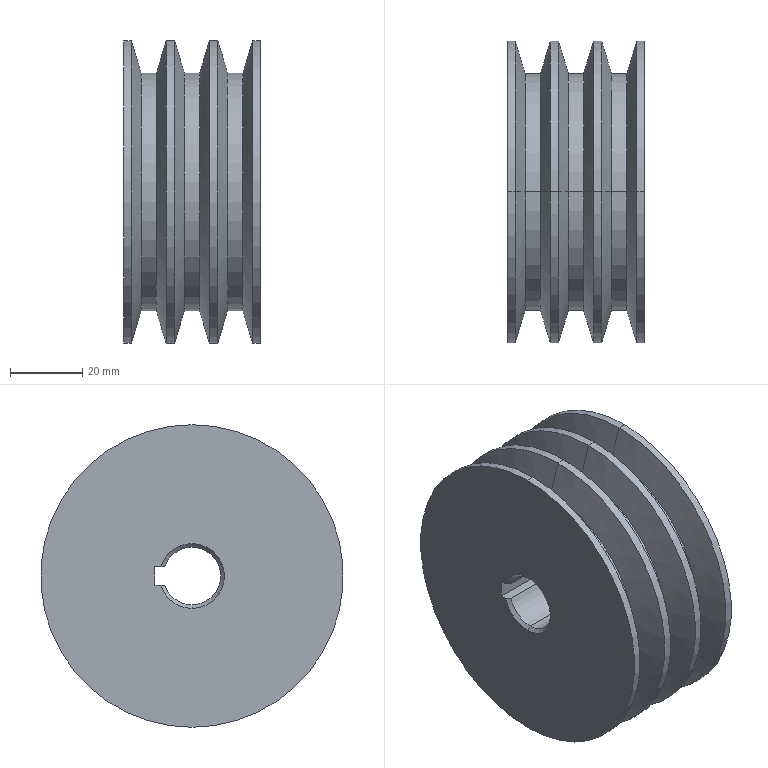Part | SolidWorks | features Chamfer 1, Cut 1, LPattern 1, RevCut 1, Revolution 1 | 1 solid | 43 faces | box 38 x 84 x 84 mm | volume 153841 mm3 | cylinder 19 | cone 18 | plane 6 | commonest cylinder face diameters 84 x8 66 x6 16 x3 32 x2
STEP:
#1=CARTESIAN_POINT('',(1.,0.,-8.));
#2=VERTEX_POINT('',#1);
#3=CARTESIAN_POINT('',(1.,0.,8.));
#4=VERTEX_POINT('',#3);
#5=CARTESIAN_POINT('',(1.,0.,0.));
#6=DIRECTION('',(-1.,0.,0.));
#7=DIRECTION('',(0.,0.,-1.));
#8=AXIS2_PLACEMENT_3D('',#5,#6,#7);
#9=CIRCLE('',#8,8.);
#10=EDGE_CURVE('',#2,#4,#9,.T.);
#11=ORIENTED_EDGE('',*,*,#10,.F.);
#12=CARTESIAN_POINT('',(0.,0.,-9.));
#13=VERTEX_POINT('',#12);
#14=CARTESIAN_POINT('',(1.,0.,-8.));
#15=DIRECTION('',(-0.7071,0.,-0.7071));
#16=VECTOR('',#15,1000.);
#17=LINE('',#14,#16);
#18=EDGE_CURVE('',#2,#13,#17,.T.);
#19=ORIENTED_EDGE('',*,*,#18,.T.);
#20=CARTESIAN_POINT('',(0.,0.,9.));
#21=VERTEX_POINT('',#20);
#22=CARTESIAN_POINT('',(0.,0.,0.));
#23=DIRECTION('',(1.,0.,0.));
#24=DIRECTION('',(0.,0.,-1.));
#25=AXIS2_PLACEMENT_3D('',#22,#23,#24);
#26=CIRCLE('',#25,9.);
#27=EDGE_CURVE('',#21,#13,#26,.T.);
#28=ORIENTED_EDGE('',*,*,#27,.F.);
#29=CARTESIAN_POINT('',(1.,0.,8.));
#30=DIRECTION('',(-0.7071,0.,0.7071));
#31=VECTOR('',#30,1000.);
#32=LINE('',#29,#31);
#33=EDGE_CURVE('',#4,#21,#32,.T.);
#34=ORIENTED_EDGE('',*,*,#33,.F.);
#35=EDGE_LOOP('',(#11,#19,#28,#34));
#36=FACE_OUTER_BOUND('',#35,.T.);
#37=CARTESIAN_POINT('',(1.,0.,0.));
#38=DIRECTION('',(-1.,0.,0.));
#39=DIRECTION('',(0.,0.,1.));
#40=AXIS2_PLACEMENT_3D('',#37,#38,#39);
#41=CONICAL_SURFACE('',#40,8.,0.7854);
#42=ADVANCED_FACE('',(#36),#41,.F.);
#43=CARTESIAN_POINT('',(1.,7.599,2.5));
#44=VERTEX_POINT('',#43);
#45=CARTESIAN_POINT('',(1.,0.,0.));
#46=DIRECTION('',(-1.,0.,0.));
#47=DIRECTION('',(0.,0.,-1.));
#48=AXIS2_PLACEMENT_3D('',#45,#46,#47);
#49=CIRCLE('',#48,8.);
#50=EDGE_CURVE('',#4,#44,#49,.T.);
#51=ORIENTED_EDGE('',*,*,#50,.F.);
#52=ORIENTED_EDGE('',*,*,#33,.T.);
#53=CARTESIAN_POINT('',(0.,8.646,2.5));
#54=VERTEX_POINT('',#53);
#55=CARTESIAN_POINT('',(0.,0.,0.));
#56=DIRECTION('',(1.,0.,0.));
#57=DIRECTION('',(0.,0.,-1.));
#58=AXIS2_PLACEMENT_3D('',#55,#56,#57);
#59=CIRCLE('',#58,9.);
#60=EDGE_CURVE('',#54,#21,#59,.T.);
#61=ORIENTED_EDGE('',*,*,#60,.F.);
#62=CARTESIAN_POINT('',(1.,7.599,2.5));
#63=CARTESIAN_POINT('',(0.6677,7.949,2.5));
#64=CARTESIAN_POINT('',(0.3343,8.298,2.5));
#65=CARTESIAN_POINT('',(0.,8.646,2.5));
#66=B_SPLINE_CURVE_WITH_KNOTS('',3,(#62,#63,#64,#65),.UNSPECIFIED.,.F.,.F.,(4,4),(0.002397,0.003844),.UNSPECIFIED.);
#67=EDGE_CURVE('',#44,#54,#66,.T.);
#68=ORIENTED_EDGE('',*,*,#67,.F.);
#69=EDGE_LOOP('',(#51,#52,#61,#68));
#70=FACE_OUTER_BOUND('',#69,.T.);
#71=CARTESIAN_POINT('',(1.,0.,0.));
#72=DIRECTION('',(-1.,0.,0.));
#73=DIRECTION('',(0.,0.,1.));
#74=AXIS2_PLACEMENT_3D('',#71,#72,#73);
#75=CONICAL_SURFACE('',#74,8.,0.7854);
#76=ADVANCED_FACE('',(#70),#75,.F.);
#77=CARTESIAN_POINT('',(31.,0.,8.));
#78=VERTEX_POINT('',#77);
#79=CARTESIAN_POINT('',(31.,0.,-8.));
#80=VERTEX_POINT('',#79);
#81=CARTESIAN_POINT('',(31.,0.,0.));
#82=DIRECTION('',(1.,0.,0.));
#83=DIRECTION('',(0.,0.,1.));
#84=AXIS2_PLACEMENT_3D('',#81,#82,#83);
#85=CIRCLE('',#84,8.);
#86=EDGE_CURVE('',#78,#80,#85,.T.);
#87=ORIENTED_EDGE('',*,*,#86,.F.);
#88=CARTESIAN_POINT('',(32.,0.,9.));
#89=VERTEX_POINT('',#88);
#90=CARTESIAN_POINT('',(32.,0.,9.));
#91=DIRECTION('',(0.7071,0.,0.7071));
#92=VECTOR('',#91,1000.);
#93=LINE('',#90,#92);
#94=EDGE_CURVE('',#78,#89,#93,.T.);
#95=ORIENTED_EDGE('',*,*,#94,.T.);
#96=CARTESIAN_POINT('',(32.,0.,-9.));
#97=VERTEX_POINT('',#96);
#98=CARTESIAN_POINT('',(32.,0.,0.));
#99=DIRECTION('',(-1.,0.,0.));
#100=DIRECTION('',(0.,0.,1.));
#101=AXIS2_PLACEMENT_3D('',#98,#99,#100);
#102=CIRCLE('',#101,9.);
#103=EDGE_CURVE('',#97,#89,#102,.T.);
#104=ORIENTED_EDGE('',*,*,#103,.F.);
#105=CARTESIAN_POINT('',(32.,0.,-9.));
#106=DIRECTION('',(0.7071,0.,-0.7071));
#107=VECTOR('',#106,1000.);
#108=LINE('',#105,#107);
#109=EDGE_CURVE('',#80,#97,#108,.T.);
#110=ORIENTED_EDGE('',*,*,#109,.F.);
#111=EDGE_LOOP('',(#87,#95,#104,#110));
#112=FACE_OUTER_BOUND('',#111,.T.);
#113=CARTESIAN_POINT('',(32.,0.,0.));
#114=DIRECTION('',(1.,0.,0.));
#115=DIRECTION('',(0.,0.,-1.));
#116=AXIS2_PLACEMENT_3D('',#113,#114,#115);
#117=CONICAL_SURFACE('',#116,9.,0.7854);
#118=ADVANCED_FACE('',(#112),#117,.F.);
#119=CARTESIAN_POINT('',(31.,7.599,-2.5));
#120=VERTEX_POINT('',#119);
#121=CARTESIAN_POINT('',(31.,0.,0.));
#122=DIRECTION('',(1.,0.,0.));
#123=DIRECTION('',(0.,0.,1.));
#124=AXIS2_PLACEMENT_3D('',#121,#122,#123);
#125=CIRCLE('',#124,8.);
#126=EDGE_CURVE('',#80,#120,#125,.T.);
#127=ORIENTED_EDGE('',*,*,#126,.F.);
#128=ORIENTED_EDGE('',*,*,#109,.T.);
#129=CARTESIAN_POINT('',(32.,8.646,-2.5));
#130=VERTEX_POINT('',#129);
#131=CARTESIAN_POINT('',(32.,0.,0.));
#132=DIRECTION('',(-1.,0.,0.));
#133=DIRECTION('',(0.,0.,1.));
#134=AXIS2_PLACEMENT_3D('',#131,#132,#133);
#135=CIRCLE('',#134,9.);
#136=EDGE_CURVE('',#130,#97,#135,.T.);
#137=ORIENTED_EDGE('',*,*,#136,.F.);
#138=CARTESIAN_POINT('',(31.,7.599,-2.5));
#139=CARTESIAN_POINT('',(31.332,7.949,-2.5));
#140=CARTESIAN_POINT('',(31.666,8.298,-2.5));
#141=CARTESIAN_POINT('',(32.,8.646,-2.5));
#142=B_SPLINE_CURVE_WITH_KNOTS('',3,(#138,#139,#140,#141),.UNSPECIFIED.,.F.,.F.,(4,4),(0.002995,0.004443),.UNSPECIFIED.);
#143=EDGE_CURVE('',#120,#130,#142,.T.);
#144=ORIENTED_EDGE('',*,*,#143,.F.);
#145=EDGE_LOOP('',(#127,#128,#137,#144));
#146=FACE_OUTER_BOUND('',#145,.T.);
#147=CARTESIAN_POINT('',(32.,0.,0.));
#148=DIRECTION('',(1.,0.,0.));
#149=DIRECTION('',(0.,0.,-1.));
#150=AXIS2_PLACEMENT_3D('',#147,#148,#149);
#151=CONICAL_SURFACE('',#150,9.,0.7854);
#152=ADVANCED_FACE('',(#146),#151,.F.);
#153=CARTESIAN_POINT('',(28.89,0.,33.));
#154=VERTEX_POINT('',#153);
#155=CARTESIAN_POINT('',(28.89,0.,-33.));
#156=VERTEX_POINT('',#155);
#157=CARTESIAN_POINT('',(28.89,0.,0.));
#158=DIRECTION('',(-1.,0.,0.));
#159=DIRECTION('',(0.,0.,1.));
#160=AXIS2_PLACEMENT_3D('',#157,#158,#159);
#161=CIRCLE('',#160,33.);
#162=EDGE_CURVE('',#154,#156,#161,.T.);
#163=ORIENTED_EDGE('',*,*,#162,.T.);
#164=CARTESIAN_POINT('',(26.139,0.,-42.));
#165=VERTEX_POINT('',#164);
#166=CARTESIAN_POINT('',(26.139,0.,-42.));
#167=DIRECTION('',(-0.2924,0.,-0.9563));
#168=VECTOR('',#167,1000.);
#169=LINE('',#166,#168);
#170=EDGE_CURVE('',#156,#165,#169,.T.);
#171=ORIENTED_EDGE('',*,*,#170,.T.);
#172=CARTESIAN_POINT('',(26.139,0.,42.));
#173=VERTEX_POINT('',#172);
#174=CARTESIAN_POINT('',(26.139,0.,0.));
#175=DIRECTION('',(-1.,0.,0.));
#176=DIRECTION('',(0.,0.,1.));
#177=AXIS2_PLACEMENT_3D('',#174,#175,#176);
#178=CIRCLE('',#177,42.);
#179=EDGE_CURVE('',#173,#165,#178,.T.);
#180=ORIENTED_EDGE('',*,*,#179,.F.);
#181=CARTESIAN_POINT('',(26.139,0.,42.));
#182=DIRECTION('',(-0.2924,0.,0.9563));
#183=VECTOR('',#182,1000.);
#184=LINE('',#181,#183);
#185=EDGE_CURVE('',#154,#173,#184,.T.);
#186=ORIENTED_EDGE('',*,*,#185,.F.);
#187=EDGE_LOOP('',(#163,#171,#180,#186));
#188=FACE_OUTER_BOUND('',#187,.T.);
#189=CARTESIAN_POINT('',(26.139,0.,0.));
#190=DIRECTION('',(-1.,0.,0.));
#191=DIRECTION('',(0.,0.,1.));
#192=AXIS2_PLACEMENT_3D('',#189,#190,#191);
#193=CONICAL_SURFACE('',#192,42.,1.274);
#194=ADVANCED_FACE('',(#188),#193,.T.);
#195=CARTESIAN_POINT('',(33.11,0.,33.));
#196=VERTEX_POINT('',#195);
#197=CARTESIAN_POINT('',(33.11,0.,-33.));
#198=VERTEX_POINT('',#197);
#199=CARTESIAN_POINT('',(33.11,0.,0.));
#200=DIRECTION('',(-1.,0.,0.));
#201=DIRECTION('',(0.,0.,1.));
#202=AXIS2_PLACEMENT_3D('',#199,#200,#201);
#203=CIRCLE('',#202,33.);
#204=EDGE_CURVE('',#196,#198,#203,.T.);
#205=ORIENTED_EDGE('',*,*,#204,.F.);
#206=CARTESIAN_POINT('',(35.861,0.,42.));
#207=VERTEX_POINT('',#206);
#208=CARTESIAN_POINT('',(33.11,0.,33.));
#209=DIRECTION('',(0.2924,0.,0.9563));
#210=VECTOR('',#209,1000.);
#211=LINE('',#208,#210);
#212=EDGE_CURVE('',#196,#207,#211,.T.);
#213=ORIENTED_EDGE('',*,*,#212,.T.);
#214=CARTESIAN_POINT('',(35.861,0.,-42.));
#215=VERTEX_POINT('',#214);
#216=CARTESIAN_POINT('',(35.861,0.,0.));
#217=DIRECTION('',(-1.,0.,0.));
#218=DIRECTION('',(0.,0.,1.));
#219=AXIS2_PLACEMENT_3D('',#216,#217,#218);
#220=CIRCLE('',#219,42.);
#221=EDGE_CURVE('',#207,#215,#220,.T.);
#222=ORIENTED_EDGE('',*,*,#221,.T.);
#223=CARTESIAN_POINT('',(33.11,0.,-33.));
#224=DIRECTION('',(0.2924,0.,-0.9563));
#225=VECTOR('',#224,1000.);
#226=LINE('',#223,#225);
#227=EDGE_CURVE('',#198,#215,#226,.T.);
#228=ORIENTED_EDGE('',*,*,#227,.F.);
#229=EDGE_LOOP('',(#205,#213,#222,#228));
#230=FACE_OUTER_BOUND('',#229,.T.);
#231=CARTESIAN_POINT('',(33.11,0.,0.));
#232=DIRECTION('',(1.,0.,0.));
#233=DIRECTION('',(0.,0.,-1.));
#234=AXIS2_PLACEMENT_3D('',#231,#232,#233);
#235=CONICAL_SURFACE('',#234,33.,1.274);
#236=ADVANCED_FACE('',(#230),#235,.T.);
#237=ORIENTED_EDGE('',*,*,#204,.T.);
#238=CARTESIAN_POINT('',(24.,0.,-33.));
#239=DIRECTION('',(-1.,0.,0.));
#240=VECTOR('',#239,1000.);
#241=LINE('',#238,#240);
#242=EDGE_CURVE('',#198,#156,#241,.T.);
#243=ORIENTED_EDGE('',*,*,#242,.T.);
#244=ORIENTED_EDGE('',*,*,#162,.F.);
#245=CARTESIAN_POINT('',(24.,0.,33.));
#246=DIRECTION('',(-1.,0.,0.));
#247=VECTOR('',#246,1000.);
#248=LINE('',#245,#247);
#249=EDGE_CURVE('',#196,#154,#248,.T.);
#250=ORIENTED_EDGE('',*,*,#249,.F.);
#251=EDGE_LOOP('',(#237,#243,#244,#250));
#252=FACE_OUTER_BOUND('',#251,.T.);
#253=CARTESIAN_POINT('',(24.,0.,0.));
#254=DIRECTION('',(-1.,0.,0.));
#255=DIRECTION('',(0.,0.,1.));
#256=AXIS2_PLACEMENT_3D('',#253,#254,#255);
#257=CYLINDRICAL_SURFACE('',#256,33.);
#258=ADVANCED_FACE('',(#252),#257,.T.);
#259=CARTESIAN_POINT('',(16.89,0.,33.));
#260=VERTEX_POINT('',#259);
#261=CARTESIAN_POINT('',(16.89,0.,-33.));
#262=VERTEX_POINT('',#261);
#263=CARTESIAN_POINT('',(16.89,0.,0.));
#264=DIRECTION('',(-1.,0.,0.));
#265=DIRECTION('',(0.,0.,1.));
#266=AXIS2_PLACEMENT_3D('',#263,#264,#265);
#267=CIRCLE('',#266,33.);
#268=EDGE_CURVE('',#260,#262,#267,.T.);
#269=ORIENTED_EDGE('',*,*,#268,.T.);
#270=CARTESIAN_POINT('',(14.139,0.,-42.));
#271=VERTEX_POINT('',#270);
#272=CARTESIAN_POINT('',(14.139,0.,-42.));
#273=DIRECTION('',(-0.2924,0.,-0.9563));
#274=VECTOR('',#273,1000.);
#275=LINE('',#272,#274);
#276=EDGE_CURVE('',#262,#271,#275,.T.);
#277=ORIENTED_EDGE('',*,*,#276,.T.);
#278=CARTESIAN_POINT('',(14.139,0.,42.));
#279=VERTEX_POINT('',#278);
#280=CARTESIAN_POINT('',(14.139,0.,0.));
#281=DIRECTION('',(-1.,0.,0.));
#282=DIRECTION('',(0.,0.,1.));
#283=AXIS2_PLACEMENT_3D('',#280,#281,#282);
#284=CIRCLE('',#283,42.);
#285=EDGE_CURVE('',#279,#271,#284,.T.);
#286=ORIENTED_EDGE('',*,*,#285,.F.);
#287=CARTESIAN_POINT('',(14.139,0.,42.));
#288=DIRECTION('',(-0.2924,0.,0.9563));
#289=VECTOR('',#288,1000.);
#290=LINE('',#287,#289);
#291=EDGE_CURVE('',#260,#279,#290,.T.);
#292=ORIENTED_EDGE('',*,*,#291,.F.);
#293=EDGE_LOOP('',(#269,#277,#286,#292));
#294=FACE_OUTER_BOUND('',#293,.T.);
#295=CARTESIAN_POINT('',(14.139,0.,0.));
#296=DIRECTION('',(-1.,0.,0.));
#297=DIRECTION('',(0.,0.,1.));
#298=AXIS2_PLACEMENT_3D('',#295,#296,#297);
#299=CONICAL_SURFACE('',#298,42.,1.274);
#300=ADVANCED_FACE('',(#294),#299,.T.);
#301=CARTESIAN_POINT('',(21.11,0.,33.));
#302=VERTEX_POINT('',#301);
#303=CARTESIAN_POINT('',(21.11,0.,-33.));
#304=VERTEX_POINT('',#303);
#305=CARTESIAN_POINT('',(21.11,0.,0.));
#306=DIRECTION('',(-1.,0.,0.));
#307=DIRECTION('',(0.,0.,1.));
#308=AXIS2_PLACEMENT_3D('',#305,#306,#307);
#309=CIRCLE('',#308,33.);
#310=EDGE_CURVE('',#302,#304,#309,.T.);
#311=ORIENTED_EDGE('',*,*,#310,.F.);
#312=CARTESIAN_POINT('',(23.861,0.,42.));
#313=VERTEX_POINT('',#312);
#314=CARTESIAN_POINT('',(21.11,0.,33.));
#315=DIRECTION('',(0.2924,0.,0.9563));
#316=VECTOR('',#315,1000.);
#317=LINE('',#314,#316);
#318=EDGE_CURVE('',#302,#313,#317,.T.);
#319=ORIENTED_EDGE('',*,*,#318,.T.);
#320=CARTESIAN_POINT('',(23.861,0.,-42.));
#321=VERTEX_POINT('',#320);
#322=CARTESIAN_POINT('',(23.861,0.,0.));
#323=DIRECTION('',(-1.,0.,0.));
#324=DIRECTION('',(0.,0.,1.));
#325=AXIS2_PLACEMENT_3D('',#322,#323,#324);
#326=CIRCLE('',#325,42.);
#327=EDGE_CURVE('',#313,#321,#326,.T.);
#328=ORIENTED_EDGE('',*,*,#327,.T.);
#329=CARTESIAN_POINT('',(21.11,0.,-33.));
#330=DIRECTION('',(0.2924,0.,-0.9563));
#331=VECTOR('',#330,1000.);
#332=LINE('',#329,#331);
#333=EDGE_CURVE('',#304,#321,#332,.T.);
#334=ORIENTED_EDGE('',*,*,#333,.F.);
#335=EDGE_LOOP('',(#311,#319,#328,#334));
#336=FACE_OUTER_BOUND('',#335,.T.);
#337=CARTESIAN_POINT('',(21.11,0.,0.));
#338=DIRECTION('',(1.,0.,0.));
#339=DIRECTION('',(0.,0.,-1.));
#340=AXIS2_PLACEMENT_3D('',#337,#338,#339);
#341=CONICAL_SURFACE('',#340,33.,1.274);
#342=ADVANCED_FACE('',(#336),#341,.T.);
#343=ORIENTED_EDGE('',*,*,#310,.T.);
#344=CARTESIAN_POINT('',(12.,0.,-33.));
#345=DIRECTION('',(-1.,0.,0.));
#346=VECTOR('',#345,1000.);
#347=LINE('',#344,#346);
#348=EDGE_CURVE('',#304,#262,#347,.T.);
#349=ORIENTED_EDGE('',*,*,#348,.T.);
#350=ORIENTED_EDGE('',*,*,#268,.F.);
#351=CARTESIAN_POINT('',(12.,0.,33.));
#352=DIRECTION('',(-1.,0.,0.));
#353=VECTOR('',#352,1000.);
#354=LINE('',#351,#353);
#355=EDGE_CURVE('',#302,#260,#354,.T.);
#356=ORIENTED_EDGE('',*,*,#355,.F.);
#357=EDGE_LOOP('',(#343,#349,#350,#356));
#358=FACE_OUTER_BOUND('',#357,.T.);
#359=CARTESIAN_POINT('',(12.,0.,0.));
#360=DIRECTION('',(-1.,0.,0.));
#361=DIRECTION('',(0.,0.,1.));
#362=AXIS2_PLACEMENT_3D('',#359,#360,#361);
#363=CYLINDRICAL_SURFACE('',#362,33.);
#364=ADVANCED_FACE('',(#358),#363,.T.);
#365=CARTESIAN_POINT('',(4.89,0.,33.));
#366=VERTEX_POINT('',#365);
#367=CARTESIAN_POINT('',(4.89,0.,-33.));
#368=VERTEX_POINT('',#367);
#369=CARTESIAN_POINT('',(4.89,0.,0.));
#370=DIRECTION('',(-1.,0.,0.));
#371=DIRECTION('',(0.,0.,1.));
#372=AXIS2_PLACEMENT_3D('',#369,#370,#371);
#373=CIRCLE('',#372,33.);
#374=EDGE_CURVE('',#366,#368,#373,.T.);
#375=ORIENTED_EDGE('',*,*,#374,.T.);
#376=CARTESIAN_POINT('',(2.139,0.,-42.));
#377=VERTEX_POINT('',#376);
#378=CARTESIAN_POINT('',(2.139,0.,-42.));
#379=DIRECTION('',(-0.2924,0.,-0.9563));
#380=VECTOR('',#379,1000.);
#381=LINE('',#378,#380);
#382=EDGE_CURVE('',#368,#377,#381,.T.);
#383=ORIENTED_EDGE('',*,*,#382,.T.);
#384=CARTESIAN_POINT('',(2.139,0.,42.));
#385=VERTEX_POINT('',#384);
#386=CARTESIAN_POINT('',(2.139,0.,0.));
#387=DIRECTION('',(-1.,0.,0.));
#388=DIRECTION('',(0.,0.,1.));
#389=AXIS2_PLACEMENT_3D('',#386,#387,#388);
#390=CIRCLE('',#389,42.);
#391=EDGE_CURVE('',#385,#377,#390,.T.);
#392=ORIENTED_EDGE('',*,*,#391,.F.);
#393=CARTESIAN_POINT('',(2.139,0.,42.));
#394=DIRECTION('',(-0.2924,0.,0.9563));
#395=VECTOR('',#394,1000.);
#396=LINE('',#393,#395);
#397=EDGE_CURVE('',#366,#385,#396,.T.);
#398=ORIENTED_EDGE('',*,*,#397,.F.);
#399=EDGE_LOOP('',(#375,#383,#392,#398));
#400=FACE_OUTER_BOUND('',#399,.T.);
#401=CARTESIAN_POINT('',(2.139,0.,0.));
#402=DIRECTION('',(-1.,0.,0.));
#403=DIRECTION('',(0.,0.,1.));
#404=AXIS2_PLACEMENT_3D('',#401,#402,#403);
#405=CONICAL_SURFACE('',#404,42.,1.274);
#406=ADVANCED_FACE('',(#400),#405,.T.);
#407=CARTESIAN_POINT('',(9.11,0.,33.));
#408=VERTEX_POINT('',#407);
#409=CARTESIAN_POINT('',(9.11,0.,-33.));
#410=VERTEX_POINT('',#409);
#411=CARTESIAN_POINT('',(9.11,0.,0.));
#412=DIRECTION('',(-1.,0.,0.));
#413=DIRECTION('',(0.,0.,1.));
#414=AXIS2_PLACEMENT_3D('',#411,#412,#413);
#415=CIRCLE('',#414,33.);
#416=EDGE_CURVE('',#408,#410,#415,.T.);
#417=ORIENTED_EDGE('',*,*,#416,.F.);
#418=CARTESIAN_POINT('',(11.861,0.,42.));
#419=VERTEX_POINT('',#418);
#420=CARTESIAN_POINT('',(9.11,0.,33.));
#421=DIRECTION('',(0.2924,0.,0.9563));
#422=VECTOR('',#421,1000.);
#423=LINE('',#420,#422);
#424=EDGE_CURVE('',#408,#419,#423,.T.);
#425=ORIENTED_EDGE('',*,*,#424,.T.);
#426=CARTESIAN_POINT('',(11.861,0.,-42.));
#427=VERTEX_POINT('',#426);
#428=CARTESIAN_POINT('',(11.861,0.,0.));
#429=DIRECTION('',(-1.,0.,0.));
#430=DIRECTION('',(0.,0.,1.));
#431=AXIS2_PLACEMENT_3D('',#428,#429,#430);
#432=CIRCLE('',#431,42.);
#433=EDGE_CURVE('',#419,#427,#432,.T.);
#434=ORIENTED_EDGE('',*,*,#433,.T.);
#435=CARTESIAN_POINT('',(9.11,0.,-33.));
#436=DIRECTION('',(0.2924,0.,-0.9563));
#437=VECTOR('',#436,1000.);
#438=LINE('',#435,#437);
#439=EDGE_CURVE('',#410,#427,#438,.T.);
#440=ORIENTED_EDGE('',*,*,#439,.F.);
#441=EDGE_LOOP('',(#417,#425,#434,#440));
#442=FACE_OUTER_BOUND('',#441,.T.);
#443=CARTESIAN_POINT('',(9.11,0.,0.));
#444=DIRECTION('',(1.,0.,0.));
#445=DIRECTION('',(0.,0.,-1.));
#446=AXIS2_PLACEMENT_3D('',#443,#444,#445);
#447=CONICAL_SURFACE('',#446,33.,1.274);
#448=ADVANCED_FACE('',(#442),#447,.T.);
#449=ORIENTED_EDGE('',*,*,#416,.T.);
#450=CARTESIAN_POINT('',(0.,0.,-33.));
#451=DIRECTION('',(-1.,0.,0.));
#452=VECTOR('',#451,1000.);
#453=LINE('',#450,#452);
#454=EDGE_CURVE('',#410,#368,#453,.T.);
#455=ORIENTED_EDGE('',*,*,#454,.T.);
#456=ORIENTED_EDGE('',*,*,#374,.F.);
#457=CARTESIAN_POINT('',(0.,0.,33.));
#458=DIRECTION('',(-1.,0.,0.));
#459=VECTOR('',#458,1000.);
#460=LINE('',#457,#459);
#461=EDGE_CURVE('',#408,#366,#460,.T.);
#462=ORIENTED_EDGE('',*,*,#461,.F.);
#463=EDGE_LOOP('',(#449,#455,#456,#462));
#464=FACE_OUTER_BOUND('',#463,.T.);
#465=CARTESIAN_POINT('',(0.,0.,0.));
#466=DIRECTION('',(-1.,0.,0.));
#467=DIRECTION('',(0.,0.,1.));
#468=AXIS2_PLACEMENT_3D('',#465,#466,#467);
#469=CYLINDRICAL_SURFACE('',#468,33.);
#470=ADVANCED_FACE('',(#464),#469,.T.);
#471=CARTESIAN_POINT('',(38.,0.,-16.));
#472=VERTEX_POINT('',#471);
#473=CARTESIAN_POINT('',(38.,0.,16.));
#474=VERTEX_POINT('',#473);
#475=CARTESIAN_POINT('',(38.,0.,0.));
#476=DIRECTION('',(-1.,0.,0.));
#477=DIRECTION('',(0.,0.,1.));
#478=AXIS2_PLACEMENT_3D('',#475,#476,#477);
#479=CIRCLE('',#478,16.);
#480=EDGE_CURVE('',#472,#474,#479,.T.);
#481=ORIENTED_EDGE('',*,*,#480,.F.);
#482=CARTESIAN_POINT('',(32.,0.,-16.));
#483=VERTEX_POINT('',#482);
#484=CARTESIAN_POINT('',(0.,0.,-16.));
#485=DIRECTION('',(-1.,0.,0.));
#486=VECTOR('',#485,1000.);
#487=LINE('',#484,#486);
#488=EDGE_CURVE('',#472,#483,#487,.T.);
#489=ORIENTED_EDGE('',*,*,#488,.T.);
#490=CARTESIAN_POINT('',(32.,0.,16.));
#491=VERTEX_POINT('',#490);
#492=CARTESIAN_POINT('',(32.,0.,0.));
#493=DIRECTION('',(-1.,0.,0.));
#494=DIRECTION('',(0.,0.,1.));
#495=AXIS2_PLACEMENT_3D('',#492,#493,#494);
#496=CIRCLE('',#495,16.);
#497=EDGE_CURVE('',#483,#491,#496,.T.);
#498=ORIENTED_EDGE('',*,*,#497,.T.);
#499=CARTESIAN_POINT('',(0.,0.,16.));
#500=DIRECTION('',(-1.,0.,0.));
#501=VECTOR('',#500,1000.);
#502=LINE('',#499,#501);
#503=EDGE_CURVE('',#474,#491,#502,.T.);
#504=ORIENTED_EDGE('',*,*,#503,.F.);
#505=EDGE_LOOP('',(#481,#489,#498,#504));
#506=FACE_OUTER_BOUND('',#505,.T.);
#507=CARTESIAN_POINT('',(0.,0.,0.));
#508=DIRECTION('',(-1.,0.,0.));
#509=DIRECTION('',(0.,0.,1.));
#510=AXIS2_PLACEMENT_3D('',#507,#508,#509);
#511=CYLINDRICAL_SURFACE('',#510,16.);
#512=ADVANCED_FACE('',(#506),#511,.F.);
#513=ORIENTED_EDGE('',*,*,#86,.T.);
#514=CARTESIAN_POINT('',(0.,0.,-8.));
#515=DIRECTION('',(-1.,0.,0.));
#516=VECTOR('',#515,1000.);
#517=LINE('',#514,#516);
#518=EDGE_CURVE('',#80,#2,#517,.T.);
#519=ORIENTED_EDGE('',*,*,#518,.T.);
#520=ORIENTED_EDGE('',*,*,#10,.T.);
#521=CARTESIAN_POINT('',(0.,0.,8.));
#522=DIRECTION('',(-1.,0.,0.));
#523=VECTOR('',#522,1000.);
#524=LINE('',#521,#523);
#525=EDGE_CURVE('',#78,#4,#524,.T.);
#526=ORIENTED_EDGE('',*,*,#525,.F.);
#527=EDGE_LOOP('',(#513,#519,#520,#526));
#528=FACE_OUTER_BOUND('',#527,.T.);
#529=CARTESIAN_POINT('',(0.,0.,0.));
#530=DIRECTION('',(-1.,0.,0.));
#531=DIRECTION('',(0.,0.,1.));
#532=AXIS2_PLACEMENT_3D('',#529,#530,#531);
#533=CYLINDRICAL_SURFACE('',#532,8.);
#534=ADVANCED_FACE('',(#528),#533,.F.);
#535=CARTESIAN_POINT('',(31.,7.599,2.5));
#536=VERTEX_POINT('',#535);
#537=CARTESIAN_POINT('',(31.,0.,0.));
#538=DIRECTION('',(1.,0.,0.));
#539=DIRECTION('',(0.,0.,1.));
#540=AXIS2_PLACEMENT_3D('',#537,#538,#539);
#541=CIRCLE('',#540,8.);
#542=EDGE_CURVE('',#536,#78,#541,.T.);
#543=ORIENTED_EDGE('',*,*,#542,.T.);
#544=ORIENTED_EDGE('',*,*,#525,.T.);
#545=ORIENTED_EDGE('',*,*,#50,.T.);
#546=CARTESIAN_POINT('',(38.,7.599,2.5));
#547=DIRECTION('',(-1.,0.,0.));
#548=VECTOR('',#547,1000.);
#549=LINE('',#546,#548);
#550=EDGE_CURVE('',#536,#44,#549,.T.);
#551=ORIENTED_EDGE('',*,*,#550,.F.);
#552=EDGE_LOOP('',(#543,#544,#545,#551));
#553=FACE_OUTER_BOUND('',#552,.T.);
#554=CARTESIAN_POINT('',(0.,0.,0.));
#555=DIRECTION('',(-1.,0.,0.));
#556=DIRECTION('',(0.,0.,1.));
#557=AXIS2_PLACEMENT_3D('',#554,#555,#556);
#558=CYLINDRICAL_SURFACE('',#557,8.);
#559=ADVANCED_FACE('',(#553),#558,.F.);
#560=ORIENTED_EDGE('',*,*,#391,.T.);
#561=CARTESIAN_POINT('',(0.,0.,-42.));
#562=VERTEX_POINT('',#561);
#563=CARTESIAN_POINT('',(0.,0.,-42.));
#564=DIRECTION('',(-1.,0.,0.));
#565=VECTOR('',#564,1000.);
#566=LINE('',#563,#565);
#567=EDGE_CURVE('',#377,#562,#566,.T.);
#568=ORIENTED_EDGE('',*,*,#567,.T.);
#569=CARTESIAN_POINT('',(0.,0.,42.));
#570=VERTEX_POINT('',#569);
#571=CARTESIAN_POINT('',(0.,0.,0.));
#572=DIRECTION('',(-1.,0.,0.));
#573=DIRECTION('',(0.,0.,1.));
#574=AXIS2_PLACEMENT_3D('',#571,#572,#573);
#575=CIRCLE('',#574,42.);
#576=EDGE_CURVE('',#570,#562,#575,.T.);
#577=ORIENTED_EDGE('',*,*,#576,.F.);
#578=CARTESIAN_POINT('',(0.,0.,42.));
#579=DIRECTION('',(-1.,0.,0.));
#580=VECTOR('',#579,1000.);
#581=LINE('',#578,#580);
#582=EDGE_CURVE('',#385,#570,#581,.T.);
#583=ORIENTED_EDGE('',*,*,#582,.F.);
#584=EDGE_LOOP('',(#560,#568,#577,#583));
#585=FACE_OUTER_BOUND('',#584,.T.);
#586=CARTESIAN_POINT('',(0.,0.,0.));
#587=DIRECTION('',(-1.,0.,0.));
#588=DIRECTION('',(0.,0.,1.));
#589=AXIS2_PLACEMENT_3D('',#586,#587,#588);
#590=CYLINDRICAL_SURFACE('',#589,42.);
#591=ADVANCED_FACE('',(#585),#590,.T.);
#592=ORIENTED_EDGE('',*,*,#285,.T.);
#593=CARTESIAN_POINT('',(0.,0.,-42.));
#594=DIRECTION('',(-1.,0.,0.));
#595=VECTOR('',#594,1000.);
#596=LINE('',#593,#595);
#597=EDGE_CURVE('',#271,#427,#596,.T.);
#598=ORIENTED_EDGE('',*,*,#597,.T.);
#599=ORIENTED_EDGE('',*,*,#433,.F.);
#600=CARTESIAN_POINT('',(0.,0.,42.));
#601=DIRECTION('',(-1.,0.,0.));
#602=VECTOR('',#601,1000.);
#603=LINE('',#600,#602);
#604=EDGE_CURVE('',#279,#419,#603,.T.);
#605=ORIENTED_EDGE('',*,*,#604,.F.);
#606=EDGE_LOOP('',(#592,#598,#599,#605));
#607=FACE_OUTER_BOUND('',#606,.T.);
#608=CARTESIAN_POINT('',(0.,0.,0.));
#609=DIRECTION('',(-1.,0.,0.));
#610=DIRECTION('',(0.,0.,1.));
#611=AXIS2_PLACEMENT_3D('',#608,#609,#610);
#612=CYLINDRICAL_SURFACE('',#611,42.);
#613=ADVANCED_FACE('',(#607),#612,.T.);
#614=ORIENTED_EDGE('',*,*,#179,.T.);
#615=CARTESIAN_POINT('',(0.,0.,-42.));
#616=DIRECTION('',(-1.,0.,0.));
#617=VECTOR('',#616,1000.);
#618=LINE('',#615,#617);
#619=EDGE_CURVE('',#165,#321,#618,.T.);
#620=ORIENTED_EDGE('',*,*,#619,.T.);
#621=ORIENTED_EDGE('',*,*,#327,.F.);
#622=CARTESIAN_POINT('',(0.,0.,42.));
#623=DIRECTION('',(-1.,0.,0.));
#624=VECTOR('',#623,1000.);
#625=LINE('',#622,#624);
#626=EDGE_CURVE('',#173,#313,#625,.T.);
#627=ORIENTED_EDGE('',*,*,#626,.F.);
#628=EDGE_LOOP('',(#614,#620,#621,#627));
#629=FACE_OUTER_BOUND('',#628,.T.);
#630=CARTESIAN_POINT('',(0.,0.,0.));
#631=DIRECTION('',(-1.,0.,0.));
#632=DIRECTION('',(0.,0.,1.));
#633=AXIS2_PLACEMENT_3D('',#630,#631,#632);
#634=CYLINDRICAL_SURFACE('',#633,42.);
#635=ADVANCED_FACE('',(#629),#634,.T.);
#636=CARTESIAN_POINT('',(38.,0.,42.));
#637=VERTEX_POINT('',#636);
#638=CARTESIAN_POINT('',(38.,0.,-42.));
#639=VERTEX_POINT('',#638);
#640=CARTESIAN_POINT('',(38.,0.,0.));
#641=DIRECTION('',(-1.,0.,0.));
#642=DIRECTION('',(0.,0.,1.));
#643=AXIS2_PLACEMENT_3D('',#640,#641,#642);
#644=CIRCLE('',#643,42.);
#645=EDGE_CURVE('',#637,#639,#644,.T.);
#646=ORIENTED_EDGE('',*,*,#645,.T.);
#647=CARTESIAN_POINT('',(0.,0.,-42.));
#648=DIRECTION('',(-1.,0.,0.));
#649=VECTOR('',#648,1000.);
#650=LINE('',#647,#649);
#651=EDGE_CURVE('',#639,#215,#650,.T.);
#652=ORIENTED_EDGE('',*,*,#651,.T.);
#653=ORIENTED_EDGE('',*,*,#221,.F.);
#654=CARTESIAN_POINT('',(0.,0.,42.));
#655=DIRECTION('',(-1.,0.,0.));
#656=VECTOR('',#655,1000.);
#657=LINE('',#654,#656);
#658=EDGE_CURVE('',#637,#207,#657,.T.);
#659=ORIENTED_EDGE('',*,*,#658,.F.);
#660=EDGE_LOOP('',(#646,#652,#653,#659));
#661=FACE_OUTER_BOUND('',#660,.T.);
#662=CARTESIAN_POINT('',(0.,0.,0.));
#663=DIRECTION('',(-1.,0.,0.));
#664=DIRECTION('',(0.,0.,1.));
#665=AXIS2_PLACEMENT_3D('',#662,#663,#664);
#666=CYLINDRICAL_SURFACE('',#665,42.);
#667=ADVANCED_FACE('',(#661),#666,.T.);
#668=ORIENTED_EDGE('',*,*,#651,.F.);
#669=CARTESIAN_POINT('',(38.,0.,0.));
#670=DIRECTION('',(-1.,0.,0.));
#671=DIRECTION('',(0.,0.,1.));
#672=AXIS2_PLACEMENT_3D('',#669,#670,#671);
#673=CIRCLE('',#672,42.);
#674=EDGE_CURVE('',#639,#637,#673,.T.);
#675=ORIENTED_EDGE('',*,*,#674,.T.);
#676=ORIENTED_EDGE('',*,*,#658,.T.);
#677=CARTESIAN_POINT('',(35.861,0.,0.));
#678=DIRECTION('',(-1.,0.,0.));
#679=DIRECTION('',(0.,0.,1.));
#680=AXIS2_PLACEMENT_3D('',#677,#678,#679);
#681=CIRCLE('',#680,42.);
#682=EDGE_CURVE('',#215,#207,#681,.T.);
#683=ORIENTED_EDGE('',*,*,#682,.F.);
#684=EDGE_LOOP('',(#668,#675,#676,#683));
#685=FACE_OUTER_BOUND('',#684,.T.);
#686=CARTESIAN_POINT('',(0.,0.,0.));
#687=DIRECTION('',(-1.,0.,0.));
#688=DIRECTION('',(0.,0.,1.));
#689=AXIS2_PLACEMENT_3D('',#686,#687,#688);
#690=CYLINDRICAL_SURFACE('',#689,42.);
#691=ADVANCED_FACE('',(#685),#690,.T.);
#692=ORIENTED_EDGE('',*,*,#619,.F.);
#693=CARTESIAN_POINT('',(26.139,0.,0.));
#694=DIRECTION('',(-1.,0.,0.));
#695=DIRECTION('',(0.,0.,1.));
#696=AXIS2_PLACEMENT_3D('',#693,#694,#695);
#697=CIRCLE('',#696,42.);
#698=EDGE_CURVE('',#165,#173,#697,.T.);
#699=ORIENTED_EDGE('',*,*,#698,.T.);
#700=ORIENTED_EDGE('',*,*,#626,.T.);
#701=CARTESIAN_POINT('',(23.861,0.,0.));
#702=DIRECTION('',(-1.,0.,0.));
#703=DIRECTION('',(0.,0.,1.));
#704=AXIS2_PLACEMENT_3D('',#701,#702,#703);
#705=CIRCLE('',#704,42.);
#706=EDGE_CURVE('',#321,#313,#705,.T.);
#707=ORIENTED_EDGE('',*,*,#706,.F.);
#708=EDGE_LOOP('',(#692,#699,#700,#707));
#709=FACE_OUTER_BOUND('',#708,.T.);
#710=CARTESIAN_POINT('',(0.,0.,0.));
#711=DIRECTION('',(-1.,0.,0.));
#712=DIRECTION('',(0.,0.,1.));
#713=AXIS2_PLACEMENT_3D('',#710,#711,#712);
#714=CYLINDRICAL_SURFACE('',#713,42.);
#715=ADVANCED_FACE('',(#709),#714,.T.);
#716=ORIENTED_EDGE('',*,*,#597,.F.);
#717=CARTESIAN_POINT('',(14.139,0.,0.));
#718=DIRECTION('',(-1.,0.,0.));
#719=DIRECTION('',(0.,0.,1.));
#720=AXIS2_PLACEMENT_3D('',#717,#718,#719);
#721=CIRCLE('',#720,42.);
#722=EDGE_CURVE('',#271,#279,#721,.T.);
#723=ORIENTED_EDGE('',*,*,#722,.T.);
#724=ORIENTED_EDGE('',*,*,#604,.T.);
#725=CARTESIAN_POINT('',(11.861,0.,0.));
#726=DIRECTION('',(-1.,0.,0.));
#727=DIRECTION('',(0.,0.,1.));
#728=AXIS2_PLACEMENT_3D('',#725,#726,#727);
#729=CIRCLE('',#728,42.);
#730=EDGE_CURVE('',#427,#419,#729,.T.);
#731=ORIENTED_EDGE('',*,*,#730,.F.);
#732=EDGE_LOOP('',(#716,#723,#724,#731));
#733=FACE_OUTER_BOUND('',#732,.T.);
#734=CARTESIAN_POINT('',(0.,0.,0.));
#735=DIRECTION('',(-1.,0.,0.));
#736=DIRECTION('',(0.,0.,1.));
#737=AXIS2_PLACEMENT_3D('',#734,#735,#736);
#738=CYLINDRICAL_SURFACE('',#737,42.);
#739=ADVANCED_FACE('',(#733),#738,.T.);
#740=ORIENTED_EDGE('',*,*,#567,.F.);
#741=CARTESIAN_POINT('',(2.139,0.,0.));
#742=DIRECTION('',(-1.,0.,0.));
#743=DIRECTION('',(0.,0.,1.));
#744=AXIS2_PLACEMENT_3D('',#741,#742,#743);
#745=CIRCLE('',#744,42.);
#746=EDGE_CURVE('',#377,#385,#745,.T.);
#747=ORIENTED_EDGE('',*,*,#746,.T.);
#748=ORIENTED_EDGE('',*,*,#582,.T.);
#749=CARTESIAN_POINT('',(0.,0.,0.));
#750=DIRECTION('',(-1.,0.,0.));
#751=DIRECTION('',(0.,0.,1.));
#752=AXIS2_PLACEMENT_3D('',#749,#750,#751);
#753=CIRCLE('',#752,42.);
#754=EDGE_CURVE('',#562,#570,#753,.T.);
#755=ORIENTED_EDGE('',*,*,#754,.F.);
#756=EDGE_LOOP('',(#740,#747,#748,#755));
#757=FACE_OUTER_BOUND('',#756,.T.);
#758=CARTESIAN_POINT('',(0.,0.,0.));
#759=DIRECTION('',(-1.,0.,0.));
#760=DIRECTION('',(0.,0.,1.));
#761=AXIS2_PLACEMENT_3D('',#758,#759,#760);
#762=CYLINDRICAL_SURFACE('',#761,42.);
#763=ADVANCED_FACE('',(#757),#762,.T.);
#764=ORIENTED_EDGE('',*,*,#518,.F.);
#765=ORIENTED_EDGE('',*,*,#126,.T.);
#766=CARTESIAN_POINT('',(1.,7.599,-2.5));
#767=VERTEX_POINT('',#766);
#768=CARTESIAN_POINT('',(38.,7.599,-2.5));
#769=DIRECTION('',(-1.,0.,0.));
#770=VECTOR('',#769,1000.);
#771=LINE('',#768,#770);
#772=EDGE_CURVE('',#120,#767,#771,.T.);
#773=ORIENTED_EDGE('',*,*,#772,.T.);
#774=CARTESIAN_POINT('',(1.,0.,0.));
#775=DIRECTION('',(-1.,0.,0.));
#776=DIRECTION('',(0.,0.,-1.));
#777=AXIS2_PLACEMENT_3D('',#774,#775,#776);
#778=CIRCLE('',#777,8.);
#779=EDGE_CURVE('',#767,#2,#778,.T.);
#780=ORIENTED_EDGE('',*,*,#779,.T.);
#781=EDGE_LOOP('',(#764,#765,#773,#780));
#782=FACE_OUTER_BOUND('',#781,.T.);
#783=CARTESIAN_POINT('',(0.,0.,0.));
#784=DIRECTION('',(-1.,0.,0.));
#785=DIRECTION('',(0.,0.,1.));
#786=AXIS2_PLACEMENT_3D('',#783,#784,#785);
#787=CYLINDRICAL_SURFACE('',#786,8.);
#788=ADVANCED_FACE('',(#782),#787,.F.);
#789=ORIENTED_EDGE('',*,*,#60,.T.);
#790=ORIENTED_EDGE('',*,*,#27,.T.);
#791=CARTESIAN_POINT('',(0.,8.646,-2.5));
#792=VERTEX_POINT('',#791);
#793=CARTESIAN_POINT('',(0.,0.,0.));
#794=DIRECTION('',(1.,0.,0.));
#795=DIRECTION('',(0.,0.,-1.));
#796=AXIS2_PLACEMENT_3D('',#793,#794,#795);
#797=CIRCLE('',#796,9.);
#798=EDGE_CURVE('',#13,#792,#797,.T.);
#799=ORIENTED_EDGE('',*,*,#798,.T.);
#800=CARTESIAN_POINT('',(0.,10.3,-2.5));
#801=VERTEX_POINT('',#800);
#802=CARTESIAN_POINT('',(0.,7.599,-2.5));
#803=DIRECTION('',(0.,-1.,0.));
#804=VECTOR('',#803,1000.);
#805=LINE('',#802,#804);
#806=EDGE_CURVE('',#801,#792,#805,.T.);
#807=ORIENTED_EDGE('',*,*,#806,.F.);
#808=CARTESIAN_POINT('',(0.,10.3,2.5));
#809=VERTEX_POINT('',#808);
#810=CARTESIAN_POINT('',(0.,10.3,-2.5));
#811=DIRECTION('',(0.,0.,-1.));
#812=VECTOR('',#811,1000.);
#813=LINE('',#810,#812);
#814=EDGE_CURVE('',#809,#801,#813,.T.);
#815=ORIENTED_EDGE('',*,*,#814,.F.);
#816=CARTESIAN_POINT('',(0.,7.599,2.5));
#817=DIRECTION('',(0.,1.,0.));
#818=VECTOR('',#817,1000.);
#819=LINE('',#816,#818);
#820=EDGE_CURVE('',#54,#809,#819,.T.);
#821=ORIENTED_EDGE('',*,*,#820,.F.);
#822=EDGE_LOOP('',(#789,#790,#799,#807,#815,#821));
#823=FACE_BOUND('',#822,.T.);
#824=ORIENTED_EDGE('',*,*,#576,.T.);
#825=ORIENTED_EDGE('',*,*,#754,.T.);
#826=EDGE_LOOP('',(#824,#825));
#827=FACE_OUTER_BOUND('',#826,.T.);
#828=CARTESIAN_POINT('',(0.,8.,0.));
#829=DIRECTION('',(1.,0.,0.));
#830=DIRECTION('',(0.,0.,-1.));
#831=AXIS2_PLACEMENT_3D('',#828,#829,#830);
#832=PLANE('',#831);
#833=ADVANCED_FACE('',(#823,#827),#832,.F.);
#834=ORIENTED_EDGE('',*,*,#645,.F.);
#835=ORIENTED_EDGE('',*,*,#674,.F.);
#836=EDGE_LOOP('',(#834,#835));
#837=FACE_OUTER_BOUND('',#836,.T.);
#838=CARTESIAN_POINT('',(38.,0.,0.));
#839=DIRECTION('',(-1.,0.,0.));
#840=DIRECTION('',(0.,0.,1.));
#841=AXIS2_PLACEMENT_3D('',#838,#839,#840);
#842=CIRCLE('',#841,16.);
#843=EDGE_CURVE('',#474,#472,#842,.T.);
#844=ORIENTED_EDGE('',*,*,#843,.T.);
#845=ORIENTED_EDGE('',*,*,#480,.T.);
#846=EDGE_LOOP('',(#844,#845));
#847=FACE_BOUND('',#846,.T.);
#848=CARTESIAN_POINT('',(38.,42.,0.));
#849=DIRECTION('',(-1.,0.,0.));
#850=DIRECTION('',(0.,0.,1.));
#851=AXIS2_PLACEMENT_3D('',#848,#849,#850);
#852=PLANE('',#851);
#853=ADVANCED_FACE('',(#837,#847),#852,.F.);
#854=ORIENTED_EDGE('',*,*,#488,.F.);
#855=ORIENTED_EDGE('',*,*,#843,.F.);
#856=ORIENTED_EDGE('',*,*,#503,.T.);
#857=CARTESIAN_POINT('',(32.,0.,0.));
#858=DIRECTION('',(-1.,0.,0.));
#859=DIRECTION('',(0.,0.,1.));
#860=AXIS2_PLACEMENT_3D('',#857,#858,#859);
#861=CIRCLE('',#860,16.);
#862=EDGE_CURVE('',#491,#483,#861,.T.);
#863=ORIENTED_EDGE('',*,*,#862,.T.);
#864=EDGE_LOOP('',(#854,#855,#856,#863));
#865=FACE_OUTER_BOUND('',#864,.T.);
#866=CARTESIAN_POINT('',(0.,0.,0.));
#867=DIRECTION('',(-1.,0.,0.));
#868=DIRECTION('',(0.,0.,1.));
#869=AXIS2_PLACEMENT_3D('',#866,#867,#868);
#870=CYLINDRICAL_SURFACE('',#869,16.);
#871=ADVANCED_FACE('',(#865),#870,.F.);
#872=CARTESIAN_POINT('',(32.,10.3,2.5));
#873=VERTEX_POINT('',#872);
#874=CARTESIAN_POINT('',(32.,10.3,-2.5));
#875=VERTEX_POINT('',#874);
#876=CARTESIAN_POINT('',(32.,10.3,0.));
#877=DIRECTION('',(0.,0.,-1.));
#878=VECTOR('',#877,1000.);
#879=LINE('',#876,#878);
#880=EDGE_CURVE('',#873,#875,#879,.T.);
#881=ORIENTED_EDGE('',*,*,#880,.T.);
#882=CARTESIAN_POINT('',(32.,16.,-2.5));
#883=DIRECTION('',(0.,-1.,0.));
#884=VECTOR('',#883,1000.);
#885=LINE('',#882,#884);
#886=EDGE_CURVE('',#875,#130,#885,.T.);
#887=ORIENTED_EDGE('',*,*,#886,.T.);
#888=ORIENTED_EDGE('',*,*,#136,.T.);
#889=ORIENTED_EDGE('',*,*,#103,.T.);
#890=CARTESIAN_POINT('',(32.,8.646,2.5));
#891=VERTEX_POINT('',#890);
#892=CARTESIAN_POINT('',(32.,0.,0.));
#893=DIRECTION('',(-1.,0.,0.));
#894=DIRECTION('',(0.,0.,1.));
#895=AXIS2_PLACEMENT_3D('',#892,#893,#894);
#896=CIRCLE('',#895,9.);
#897=EDGE_CURVE('',#89,#891,#896,.T.);
#898=ORIENTED_EDGE('',*,*,#897,.T.);
#899=CARTESIAN_POINT('',(32.,16.,2.5));
#900=DIRECTION('',(0.,1.,0.));
#901=VECTOR('',#900,1000.);
#902=LINE('',#899,#901);
#903=EDGE_CURVE('',#891,#873,#902,.T.);
#904=ORIENTED_EDGE('',*,*,#903,.T.);
#905=EDGE_LOOP('',(#881,#887,#888,#889,#898,#904));
#906=FACE_BOUND('',#905,.T.);
#907=ORIENTED_EDGE('',*,*,#862,.F.);
#908=ORIENTED_EDGE('',*,*,#497,.F.);
#909=EDGE_LOOP('',(#907,#908));
#910=FACE_OUTER_BOUND('',#909,.T.);
#911=CARTESIAN_POINT('',(32.,16.,0.));
#912=DIRECTION('',(-1.,0.,0.));
#913=DIRECTION('',(0.,0.,1.));
#914=AXIS2_PLACEMENT_3D('',#911,#912,#913);
#915=PLANE('',#914);
#916=ADVANCED_FACE('',(#906,#910),#915,.F.);
#917=ORIENTED_EDGE('',*,*,#454,.F.);
#918=CARTESIAN_POINT('',(9.11,0.,0.));
#919=DIRECTION('',(-1.,0.,0.));
#920=DIRECTION('',(0.,0.,1.));
#921=AXIS2_PLACEMENT_3D('',#918,#919,#920);
#922=CIRCLE('',#921,33.);
#923=EDGE_CURVE('',#410,#408,#922,.T.);
#924=ORIENTED_EDGE('',*,*,#923,.T.);
#925=ORIENTED_EDGE('',*,*,#461,.T.);
#926=CARTESIAN_POINT('',(4.89,0.,0.));
#927=DIRECTION('',(-1.,0.,0.));
#928=DIRECTION('',(0.,0.,1.));
#929=AXIS2_PLACEMENT_3D('',#926,#927,#928);
#930=CIRCLE('',#929,33.);
#931=EDGE_CURVE('',#368,#366,#930,.T.);
#932=ORIENTED_EDGE('',*,*,#931,.F.);
#933=EDGE_LOOP('',(#917,#924,#925,#932));
#934=FACE_OUTER_BOUND('',#933,.T.);
#935=CARTESIAN_POINT('',(0.,0.,0.));
#936=DIRECTION('',(-1.,0.,0.));
#937=DIRECTION('',(0.,0.,1.));
#938=AXIS2_PLACEMENT_3D('',#935,#936,#937);
#939=CYLINDRICAL_SURFACE('',#938,33.);
#940=ADVANCED_FACE('',(#934),#939,.T.);
#941=ORIENTED_EDGE('',*,*,#424,.F.);
#942=ORIENTED_EDGE('',*,*,#923,.F.);
#943=ORIENTED_EDGE('',*,*,#439,.T.);
#944=ORIENTED_EDGE('',*,*,#730,.T.);
#945=EDGE_LOOP('',(#941,#942,#943,#944));
#946=FACE_OUTER_BOUND('',#945,.T.);
#947=CARTESIAN_POINT('',(9.11,0.,0.));
#948=DIRECTION('',(1.,0.,0.));
#949=DIRECTION('',(0.,0.,-1.));
#950=AXIS2_PLACEMENT_3D('',#947,#948,#949);
#951=CONICAL_SURFACE('',#950,33.,1.274);
#952=ADVANCED_FACE('',(#946),#951,.T.);
#953=ORIENTED_EDGE('',*,*,#382,.F.);
#954=ORIENTED_EDGE('',*,*,#931,.T.);
#955=ORIENTED_EDGE('',*,*,#397,.T.);
#956=ORIENTED_EDGE('',*,*,#746,.F.);
#957=EDGE_LOOP('',(#953,#954,#955,#956));
#958=FACE_OUTER_BOUND('',#957,.T.);
#959=CARTESIAN_POINT('',(2.139,0.,0.));
#960=DIRECTION('',(-1.,0.,0.));
#961=DIRECTION('',(0.,0.,1.));
#962=AXIS2_PLACEMENT_3D('',#959,#960,#961);
#963=CONICAL_SURFACE('',#962,42.,1.274);
#964=ADVANCED_FACE('',(#958),#963,.T.);
#965=ORIENTED_EDGE('',*,*,#348,.F.);
#966=CARTESIAN_POINT('',(21.11,0.,0.));
#967=DIRECTION('',(-1.,0.,0.));
#968=DIRECTION('',(0.,0.,1.));
#969=AXIS2_PLACEMENT_3D('',#966,#967,#968);
#970=CIRCLE('',#969,33.);
#971=EDGE_CURVE('',#304,#302,#970,.T.);
#972=ORIENTED_EDGE('',*,*,#971,.T.);
#973=ORIENTED_EDGE('',*,*,#355,.T.);
#974=CARTESIAN_POINT('',(16.89,0.,0.));
#975=DIRECTION('',(-1.,0.,0.));
#976=DIRECTION('',(0.,0.,1.));
#977=AXIS2_PLACEMENT_3D('',#974,#975,#976);
#978=CIRCLE('',#977,33.);
#979=EDGE_CURVE('',#262,#260,#978,.T.);
#980=ORIENTED_EDGE('',*,*,#979,.F.);
#981=EDGE_LOOP('',(#965,#972,#973,#980));
#982=FACE_OUTER_BOUND('',#981,.T.);
#983=CARTESIAN_POINT('',(12.,0.,0.));
#984=DIRECTION('',(-1.,0.,0.));
#985=DIRECTION('',(0.,0.,1.));
#986=AXIS2_PLACEMENT_3D('',#983,#984,#985);
#987=CYLINDRICAL_SURFACE('',#986,33.);
#988=ADVANCED_FACE('',(#982),#987,.T.);
#989=ORIENTED_EDGE('',*,*,#318,.F.);
#990=ORIENTED_EDGE('',*,*,#971,.F.);
#991=ORIENTED_EDGE('',*,*,#333,.T.);
#992=ORIENTED_EDGE('',*,*,#706,.T.);
#993=EDGE_LOOP('',(#989,#990,#991,#992));
#994=FACE_OUTER_BOUND('',#993,.T.);
#995=CARTESIAN_POINT('',(21.11,0.,0.));
#996=DIRECTION('',(1.,0.,0.));
#997=DIRECTION('',(0.,0.,-1.));
#998=AXIS2_PLACEMENT_3D('',#995,#996,#997);
#999=CONICAL_SURFACE('',#998,33.,1.274);
#1000=ADVANCED_FACE('',(#994),#999,.T.);
#1001=ORIENTED_EDGE('',*,*,#276,.F.);
#1002=ORIENTED_EDGE('',*,*,#979,.T.);
#1003=ORIENTED_EDGE('',*,*,#291,.T.);
#1004=ORIENTED_EDGE('',*,*,#722,.F.);
#1005=EDGE_LOOP('',(#1001,#1002,#1003,#1004));
#1006=FACE_OUTER_BOUND('',#1005,.T.);
#1007=CARTESIAN_POINT('',(14.139,0.,0.));
#1008=DIRECTION('',(-1.,0.,0.));
#1009=DIRECTION('',(0.,0.,1.));
#1010=AXIS2_PLACEMENT_3D('',#1007,#1008,#1009);
#1011=CONICAL_SURFACE('',#1010,42.,1.274);
#1012=ADVANCED_FACE('',(#1006),#1011,.T.);
#1013=ORIENTED_EDGE('',*,*,#242,.F.);
#1014=CARTESIAN_POINT('',(33.11,0.,0.));
#1015=DIRECTION('',(-1.,0.,0.));
#1016=DIRECTION('',(0.,0.,1.));
#1017=AXIS2_PLACEMENT_3D('',#1014,#1015,#1016);
#1018=CIRCLE('',#1017,33.);
#1019=EDGE_CURVE('',#198,#196,#1018,.T.);
#1020=ORIENTED_EDGE('',*,*,#1019,.T.);
#1021=ORIENTED_EDGE('',*,*,#249,.T.);
#1022=CARTESIAN_POINT('',(28.89,0.,0.));
#1023=DIRECTION('',(-1.,0.,0.));
#1024=DIRECTION('',(0.,0.,1.));
#1025=AXIS2_PLACEMENT_3D('',#1022,#1023,#1024);
#1026=CIRCLE('',#1025,33.);
#1027=EDGE_CURVE('',#156,#154,#1026,.T.);
#1028=ORIENTED_EDGE('',*,*,#1027,.F.);
#1029=EDGE_LOOP('',(#1013,#1020,#1021,#1028));
#1030=FACE_OUTER_BOUND('',#1029,.T.);
#1031=CARTESIAN_POINT('',(24.,0.,0.));
#1032=DIRECTION('',(-1.,0.,0.));
#1033=DIRECTION('',(0.,0.,1.));
#1034=AXIS2_PLACEMENT_3D('',#1031,#1032,#1033);
#1035=CYLINDRICAL_SURFACE('',#1034,33.);
#1036=ADVANCED_FACE('',(#1030),#1035,.T.);
#1037=ORIENTED_EDGE('',*,*,#212,.F.);
#1038=ORIENTED_EDGE('',*,*,#1019,.F.);
#1039=ORIENTED_EDGE('',*,*,#227,.T.);
#1040=ORIENTED_EDGE('',*,*,#682,.T.);
#1041=EDGE_LOOP('',(#1037,#1038,#1039,#1040));
#1042=FACE_OUTER_BOUND('',#1041,.T.);
#1043=CARTESIAN_POINT('',(33.11,0.,0.));
#1044=DIRECTION('',(1.,0.,0.));
#1045=DIRECTION('',(0.,0.,-1.));
#1046=AXIS2_PLACEMENT_3D('',#1043,#1044,#1045);
#1047=CONICAL_SURFACE('',#1046,33.,1.274);
#1048=ADVANCED_FACE('',(#1042),#1047,.T.);
#1049=ORIENTED_EDGE('',*,*,#170,.F.);
#1050=ORIENTED_EDGE('',*,*,#1027,.T.);
#1051=ORIENTED_EDGE('',*,*,#185,.T.);
#1052=ORIENTED_EDGE('',*,*,#698,.F.);
#1053=EDGE_LOOP('',(#1049,#1050,#1051,#1052));
#1054=FACE_OUTER_BOUND('',#1053,.T.);
#1055=CARTESIAN_POINT('',(26.139,0.,0.));
#1056=DIRECTION('',(-1.,0.,0.));
#1057=DIRECTION('',(0.,0.,1.));
#1058=AXIS2_PLACEMENT_3D('',#1055,#1056,#1057);
#1059=CONICAL_SURFACE('',#1058,42.,1.274);
#1060=ADVANCED_FACE('',(#1054),#1059,.T.);
#1061=ORIENTED_EDGE('',*,*,#94,.F.);
#1062=ORIENTED_EDGE('',*,*,#542,.F.);
#1063=CARTESIAN_POINT('',(32.,8.646,2.5));
#1064=CARTESIAN_POINT('',(31.666,8.298,2.5));
#1065=CARTESIAN_POINT('',(31.332,7.949,2.5));
#1066=CARTESIAN_POINT('',(31.,7.599,2.5));
#1067=B_SPLINE_CURVE_WITH_KNOTS('',3,(#1063,#1064,#1065,#1066),.UNSPECIFIED.,.F.,.F.,(4,4),(0.002146,0.003594),.UNSPECIFIED.);
#1068=EDGE_CURVE('',#891,#536,#1067,.T.);
#1069=ORIENTED_EDGE('',*,*,#1068,.F.);
#1070=ORIENTED_EDGE('',*,*,#897,.F.);
#1071=EDGE_LOOP('',(#1061,#1062,#1069,#1070));
#1072=FACE_OUTER_BOUND('',#1071,.T.);
#1073=CARTESIAN_POINT('',(32.,0.,0.));
#1074=DIRECTION('',(1.,0.,0.));
#1075=DIRECTION('',(0.,0.,-1.));
#1076=AXIS2_PLACEMENT_3D('',#1073,#1074,#1075);
#1077=CONICAL_SURFACE('',#1076,9.,0.7854);
#1078=ADVANCED_FACE('',(#1072),#1077,.F.);
#1079=ORIENTED_EDGE('',*,*,#18,.F.);
#1080=ORIENTED_EDGE('',*,*,#779,.F.);
#1081=CARTESIAN_POINT('',(0.,8.646,-2.5));
#1082=CARTESIAN_POINT('',(0.3343,8.298,-2.5));
#1083=CARTESIAN_POINT('',(0.6677,7.949,-2.5));
#1084=CARTESIAN_POINT('',(1.,7.599,-2.5));
#1085=B_SPLINE_CURVE_WITH_KNOTS('',3,(#1081,#1082,#1083,#1084),.UNSPECIFIED.,.F.,.F.,(4,4),(0.002745,0.004192),.UNSPECIFIED.);
#1086=EDGE_CURVE('',#792,#767,#1085,.T.);
#1087=ORIENTED_EDGE('',*,*,#1086,.F.);
#1088=ORIENTED_EDGE('',*,*,#798,.F.);
#1089=EDGE_LOOP('',(#1079,#1080,#1087,#1088));
#1090=FACE_OUTER_BOUND('',#1089,.T.);
#1091=CARTESIAN_POINT('',(1.,0.,0.));
#1092=DIRECTION('',(-1.,0.,0.));
#1093=DIRECTION('',(0.,0.,1.));
#1094=AXIS2_PLACEMENT_3D('',#1091,#1092,#1093);
#1095=CONICAL_SURFACE('',#1094,8.,0.7854);
#1096=ADVANCED_FACE('',(#1090),#1095,.F.);
#1097=CARTESIAN_POINT('',(38.,10.3,2.5));
#1098=DIRECTION('',(-1.,0.,0.));
#1099=VECTOR('',#1098,1000.);
#1100=LINE('',#1097,#1099);
#1101=EDGE_CURVE('',#873,#809,#1100,.T.);
#1102=ORIENTED_EDGE('',*,*,#1101,.T.);
#1103=ORIENTED_EDGE('',*,*,#814,.T.);
#1104=CARTESIAN_POINT('',(38.,10.3,-2.5));
#1105=DIRECTION('',(-1.,0.,0.));
#1106=VECTOR('',#1105,1000.);
#1107=LINE('',#1104,#1106);
#1108=EDGE_CURVE('',#875,#801,#1107,.T.);
#1109=ORIENTED_EDGE('',*,*,#1108,.F.);
#1110=ORIENTED_EDGE('',*,*,#880,.F.);
#1111=EDGE_LOOP('',(#1102,#1103,#1109,#1110));
#1112=FACE_OUTER_BOUND('',#1111,.T.);
#1113=CARTESIAN_POINT('',(38.,10.3,-2.5));
#1114=DIRECTION('',(0.,1.,0.));
#1115=DIRECTION('',(0.,0.,1.));
#1116=AXIS2_PLACEMENT_3D('',#1113,#1114,#1115);
#1117=PLANE('',#1116);
#1118=ADVANCED_FACE('',(#1112),#1117,.F.);
#1119=ORIENTED_EDGE('',*,*,#1108,.T.);
#1120=ORIENTED_EDGE('',*,*,#806,.T.);
#1121=ORIENTED_EDGE('',*,*,#1086,.T.);
#1122=ORIENTED_EDGE('',*,*,#772,.F.);
#1123=ORIENTED_EDGE('',*,*,#143,.T.);
#1124=ORIENTED_EDGE('',*,*,#886,.F.);
#1125=EDGE_LOOP('',(#1119,#1120,#1121,#1122,#1123,#1124));
#1126=FACE_OUTER_BOUND('',#1125,.T.);
#1127=CARTESIAN_POINT('',(38.,7.599,-2.5));
#1128=DIRECTION('',(0.,0.,-1.));
#1129=DIRECTION('',(-1.,0.,0.));
#1130=AXIS2_PLACEMENT_3D('',#1127,#1128,#1129);
#1131=PLANE('',#1130);
#1132=ADVANCED_FACE('',(#1126),#1131,.F.);
#1133=ORIENTED_EDGE('',*,*,#1068,.T.);
#1134=ORIENTED_EDGE('',*,*,#550,.T.);
#1135=ORIENTED_EDGE('',*,*,#67,.T.);
#1136=ORIENTED_EDGE('',*,*,#820,.T.);
#1137=ORIENTED_EDGE('',*,*,#1101,.F.);
#1138=ORIENTED_EDGE('',*,*,#903,.F.);
#1139=EDGE_LOOP('',(#1133,#1134,#1135,#1136,#1137,#1138));
#1140=FACE_OUTER_BOUND('',#1139,.T.);
#1141=CARTESIAN_POINT('',(38.,7.599,2.5));
#1142=DIRECTION('',(0.,0.,1.));
#1143=DIRECTION('',(1.,0.,0.));
#1144=AXIS2_PLACEMENT_3D('',#1141,#1142,#1143);
#1145=PLANE('',#1144);
#1146=ADVANCED_FACE('',(#1140),#1145,.F.);
#1147=CLOSED_SHELL('',(#42,#76,#118,#152,#194,#236,#258,#300,#342,#364,#406,#448,#470,#512,#534,#559,#591,#613,#635,#667,#691,#715,#739,#763,#788,#833,#853,#871,#916,#940,#952,#964,#988,#1000,#1012,#1036,#1048,#1060,#1078,#1096,#1118,#1132,#1146));
#1148=MANIFOLD_SOLID_BREP('',#1147);
#1149=CARTESIAN_POINT('',(0.,0.,0.));
#1150=DIRECTION('',(0.,0.,1.));
#1151=DIRECTION('',(1.,0.,0.));
#1152=AXIS2_PLACEMENT_3D('',#1149,#1150,#1151);
#1153=(LENGTH_UNIT()NAMED_UNIT(*)SI_UNIT(.MILLI.,.METRE.));
#1154=UNCERTAINTY_MEASURE_WITH_UNIT(LENGTH_MEASURE(0.00001),#1153,'','');
#1155=(NAMED_UNIT(*)PLANE_ANGLE_UNIT()SI_UNIT($,.RADIAN.));
#1156=(NAMED_UNIT(*)SI_UNIT($,.STERADIAN.)SOLID_ANGLE_UNIT());
#1157=(GEOMETRIC_REPRESENTATION_CONTEXT(3)GLOBAL_UNCERTAINTY_ASSIGNED_CONTEXT((#1154))GLOBAL_UNIT_ASSIGNED_CONTEXT((#1153,#1155,#1156))REPRESENTATION_CONTEXT('',''));
#1158=ADVANCED_BREP_SHAPE_REPRESENTATION('',(#1148,#1152),#1157);